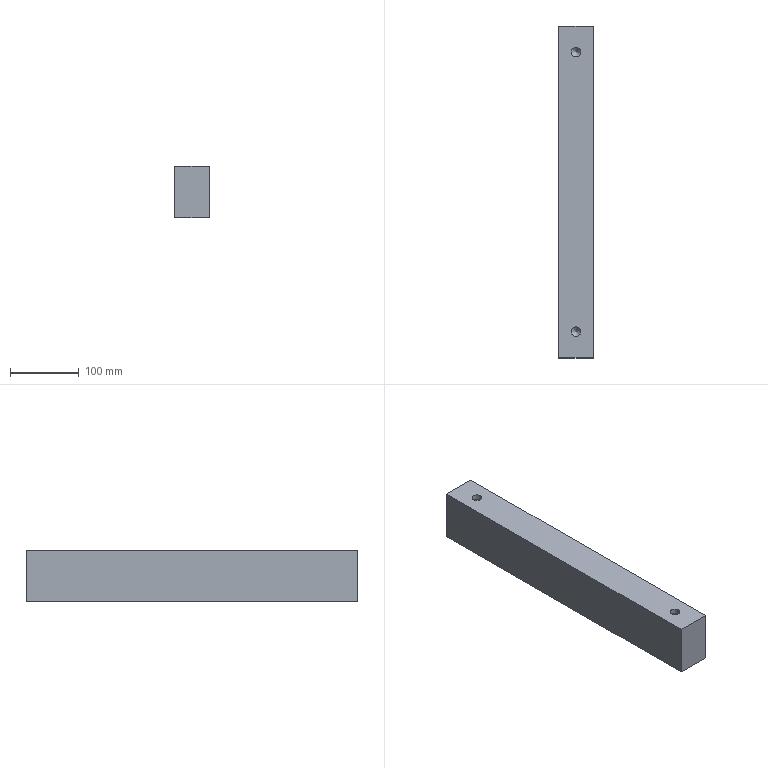Part | NX | features 3 2 | 1 solid | 10 faces | box 50 x 482.437 x 75.5 mm | volume 1817981 mm3 | plane 6 | cylinder 2 | cone 2 | commonest cylinder face diameters 14.1 x2
STEP:
#1=CARTESIAN_POINT('',(57.05,203.218,256.5));
#2=VERTEX_POINT('',#1);
#3=CARTESIAN_POINT('',(50.,203.218,256.5));
#4=DIRECTION('',(0.,0.,-1.));
#5=DIRECTION('',(1.,0.,0.));
#6=AXIS2_PLACEMENT_3D('',#3,#4,#5);
#7=CIRCLE('',#6,7.05);
#8=EDGE_CURVE('',#2,#2,#7,.T.);
#9=ORIENTED_EDGE('',*,*,#8,.T.);
#10=EDGE_LOOP('',(#9));
#11=FACE_BOUND('',#10,.T.);
#12=CARTESIAN_POINT('',(75.,241.218,256.5));
#13=VERTEX_POINT('',#12);
#14=CARTESIAN_POINT('',(75.,-241.218,256.5));
#15=VERTEX_POINT('',#14);
#16=CARTESIAN_POINT('',(75.,193.,256.5));
#17=DIRECTION('',(0.,-1.,0.));
#18=VECTOR('',#17,1000.);
#19=LINE('',#16,#18);
#20=EDGE_CURVE('',#13,#15,#19,.T.);
#21=ORIENTED_EDGE('',*,*,#20,.F.);
#22=CARTESIAN_POINT('',(25.,241.218,256.5));
#23=VERTEX_POINT('',#22);
#24=CARTESIAN_POINT('',(2065.,241.218,256.5));
#25=DIRECTION('',(1.,0.,0.));
#26=VECTOR('',#25,1000.);
#27=LINE('',#24,#26);
#28=EDGE_CURVE('',#23,#13,#27,.T.);
#29=ORIENTED_EDGE('',*,*,#28,.F.);
#30=CARTESIAN_POINT('',(25.,-241.218,256.5));
#31=VERTEX_POINT('',#30);
#32=CARTESIAN_POINT('',(25.,193.,256.5));
#33=DIRECTION('',(0.,1.,0.));
#34=VECTOR('',#33,1000.);
#35=LINE('',#32,#34);
#36=EDGE_CURVE('',#31,#23,#35,.T.);
#37=ORIENTED_EDGE('',*,*,#36,.F.);
#38=CARTESIAN_POINT('',(2065.,-241.218,256.5));
#39=DIRECTION('',(1.,0.,0.));
#40=VECTOR('',#39,1000.);
#41=LINE('',#38,#40);
#42=EDGE_CURVE('',#31,#15,#41,.T.);
#43=ORIENTED_EDGE('',*,*,#42,.T.);
#44=EDGE_LOOP('',(#21,#29,#37,#43));
#45=FACE_BOUND('',#44,.T.);
#46=CARTESIAN_POINT('',(57.05,-203.218,256.5));
#47=VERTEX_POINT('',#46);
#48=CARTESIAN_POINT('',(50.,-203.218,256.5));
#49=DIRECTION('',(0.,0.,-1.));
#50=DIRECTION('',(1.,0.,0.));
#51=AXIS2_PLACEMENT_3D('',#48,#49,#50);
#52=CIRCLE('',#51,7.05);
#53=EDGE_CURVE('',#47,#47,#52,.T.);
#54=ORIENTED_EDGE('',*,*,#53,.T.);
#55=EDGE_LOOP('',(#54));
#56=FACE_BOUND('',#55,.T.);
#57=CARTESIAN_POINT('',(2065.,0.,256.5));
#58=DIRECTION('',(0.,0.,1.));
#59=DIRECTION('',(-1.,0.,0.));
#60=AXIS2_PLACEMENT_3D('',#57,#58,#59);
#61=PLANE('',#60);
#62=ADVANCED_FACE('',(#11,#45,#56),#61,.T.);
#63=ORIENTED_EDGE('',*,*,#36,.T.);
#64=CARTESIAN_POINT('',(25.,241.218,181.));
#65=VERTEX_POINT('',#64);
#66=CARTESIAN_POINT('',(25.,241.218,-1.5));
#67=DIRECTION('',(0.,0.,1.));
#68=VECTOR('',#67,1000.);
#69=LINE('',#66,#68);
#70=EDGE_CURVE('',#65,#23,#69,.T.);
#71=ORIENTED_EDGE('',*,*,#70,.F.);
#72=CARTESIAN_POINT('',(25.,-241.218,181.));
#73=VERTEX_POINT('',#72);
#74=CARTESIAN_POINT('',(25.,193.,181.));
#75=DIRECTION('',(0.,-1.,0.));
#76=VECTOR('',#75,1000.);
#77=LINE('',#74,#76);
#78=EDGE_CURVE('',#65,#73,#77,.T.);
#79=ORIENTED_EDGE('',*,*,#78,.T.);
#80=CARTESIAN_POINT('',(25.,-241.218,-1.5));
#81=DIRECTION('',(0.,0.,1.));
#82=VECTOR('',#81,1000.);
#83=LINE('',#80,#82);
#84=EDGE_CURVE('',#73,#31,#83,.T.);
#85=ORIENTED_EDGE('',*,*,#84,.T.);
#86=EDGE_LOOP('',(#63,#71,#79,#85));
#87=FACE_BOUND('',#86,.T.);
#88=CARTESIAN_POINT('',(25.,193.,-1.5));
#89=DIRECTION('',(-1.,0.,0.));
#90=DIRECTION('',(0.,0.,-1.));
#91=AXIS2_PLACEMENT_3D('',#88,#89,#90);
#92=PLANE('',#91);
#93=ADVANCED_FACE('',(#87),#92,.T.);
#94=CARTESIAN_POINT('',(75.,-241.218,181.));
#95=VERTEX_POINT('',#94);
#96=CARTESIAN_POINT('',(75.,241.218,181.));
#97=VERTEX_POINT('',#96);
#98=CARTESIAN_POINT('',(75.,193.,181.));
#99=DIRECTION('',(0.,1.,0.));
#100=VECTOR('',#99,1000.);
#101=LINE('',#98,#100);
#102=EDGE_CURVE('',#95,#97,#101,.T.);
#103=ORIENTED_EDGE('',*,*,#102,.T.);
#104=CARTESIAN_POINT('',(75.,241.218,-1.5));
#105=DIRECTION('',(0.,0.,-1.));
#106=VECTOR('',#105,1000.);
#107=LINE('',#104,#106);
#108=EDGE_CURVE('',#13,#97,#107,.T.);
#109=ORIENTED_EDGE('',*,*,#108,.F.);
#110=ORIENTED_EDGE('',*,*,#20,.T.);
#111=CARTESIAN_POINT('',(75.,-241.218,-1.5));
#112=DIRECTION('',(0.,0.,-1.));
#113=VECTOR('',#112,1000.);
#114=LINE('',#111,#113);
#115=EDGE_CURVE('',#15,#95,#114,.T.);
#116=ORIENTED_EDGE('',*,*,#115,.T.);
#117=EDGE_LOOP('',(#103,#109,#110,#116));
#118=FACE_BOUND('',#117,.T.);
#119=CARTESIAN_POINT('',(75.,193.,-1.5));
#120=DIRECTION('',(1.,0.,0.));
#121=DIRECTION('',(0.,0.,1.));
#122=AXIS2_PLACEMENT_3D('',#119,#120,#121);
#123=PLANE('',#122);
#124=ADVANCED_FACE('',(#118),#123,.T.);
#125=ORIENTED_EDGE('',*,*,#78,.F.);
#126=CARTESIAN_POINT('',(1295.,241.218,181.));
#127=DIRECTION('',(-1.,0.,0.));
#128=VECTOR('',#127,1000.);
#129=LINE('',#126,#128);
#130=EDGE_CURVE('',#97,#65,#129,.T.);
#131=ORIENTED_EDGE('',*,*,#130,.F.);
#132=ORIENTED_EDGE('',*,*,#102,.F.);
#133=CARTESIAN_POINT('',(1295.,-241.218,181.));
#134=DIRECTION('',(-1.,0.,0.));
#135=VECTOR('',#134,1000.);
#136=LINE('',#133,#135);
#137=EDGE_CURVE('',#95,#73,#136,.T.);
#138=ORIENTED_EDGE('',*,*,#137,.T.);
#139=EDGE_LOOP('',(#125,#131,#132,#138));
#140=FACE_BOUND('',#139,.T.);
#141=CARTESIAN_POINT('',(1295.,193.,181.));
#142=DIRECTION('',(0.,0.,-1.));
#143=DIRECTION('',(-1.,0.,0.));
#144=AXIS2_PLACEMENT_3D('',#141,#142,#143);
#145=PLANE('',#144);
#146=ADVANCED_FACE('',(#140),#145,.T.);
#147=ORIENTED_EDGE('',*,*,#42,.F.);
#148=ORIENTED_EDGE('',*,*,#84,.F.);
#149=ORIENTED_EDGE('',*,*,#137,.F.);
#150=ORIENTED_EDGE('',*,*,#115,.F.);
#151=EDGE_LOOP('',(#147,#148,#149,#150));
#152=FACE_BOUND('',#151,.T.);
#153=CARTESIAN_POINT('',(-126.629,-241.218,0.));
#154=DIRECTION('',(0.,-1.,0.));
#155=DIRECTION('',(0.,0.,1.));
#156=AXIS2_PLACEMENT_3D('',#153,#154,#155);
#157=PLANE('',#156);
#158=ADVANCED_FACE('',(#152),#157,.T.);
#159=ORIENTED_EDGE('',*,*,#28,.T.);
#160=ORIENTED_EDGE('',*,*,#108,.T.);
#161=ORIENTED_EDGE('',*,*,#130,.T.);
#162=ORIENTED_EDGE('',*,*,#70,.T.);
#163=EDGE_LOOP('',(#159,#160,#161,#162));
#164=FACE_BOUND('',#163,.T.);
#165=CARTESIAN_POINT('',(-126.629,241.218,0.));
#166=DIRECTION('',(0.,1.,0.));
#167=DIRECTION('',(0.,0.,1.));
#168=AXIS2_PLACEMENT_3D('',#165,#166,#167);
#169=PLANE('',#168);
#170=ADVANCED_FACE('',(#164),#169,.T.);
#171=CARTESIAN_POINT('',(42.95,203.218,248.55));
#172=VERTEX_POINT('',#171);
#173=CARTESIAN_POINT('',(50.,203.218,248.55));
#174=DIRECTION('',(0.,0.,-1.));
#175=DIRECTION('',(-1.,0.,0.));
#176=AXIS2_PLACEMENT_3D('',#173,#174,#175);
#177=CIRCLE('',#176,7.05);
#178=EDGE_CURVE('',#172,#172,#177,.T.);
#179=ORIENTED_EDGE('',*,*,#178,.T.);
#180=EDGE_LOOP('',(#179));
#181=FACE_BOUND('',#180,.T.);
#182=ORIENTED_EDGE('',*,*,#8,.F.);
#183=EDGE_LOOP('',(#182));
#184=FACE_BOUND('',#183,.T.);
#185=CARTESIAN_POINT('',(50.,203.218,256.5));
#186=DIRECTION('',(0.,0.,-1.));
#187=DIRECTION('',(-1.,0.,0.));
#188=AXIS2_PLACEMENT_3D('',#185,#186,#187);
#189=CYLINDRICAL_SURFACE('',#188,7.05);
#190=ADVANCED_FACE('',(#181,#184),#189,.F.);
#191=CARTESIAN_POINT('',(50.,203.218,241.5));
#192=VERTEX_POINT('',#191);
#193=VERTEX_LOOP('',#192);
#194=FACE_BOUND('',#193,.T.);
#195=ORIENTED_EDGE('',*,*,#178,.F.);
#196=EDGE_LOOP('',(#195));
#197=FACE_BOUND('',#196,.T.);
#198=CARTESIAN_POINT('',(50.,203.218,248.55));
#199=DIRECTION('',(0.,0.,1.));
#200=DIRECTION('',(-1.,0.,0.));
#201=AXIS2_PLACEMENT_3D('',#198,#199,#200);
#202=CONICAL_SURFACE('',#201,7.05,0.7854);
#203=ADVANCED_FACE('',(#194,#197),#202,.F.);
#204=CARTESIAN_POINT('',(42.95,-203.218,248.55));
#205=VERTEX_POINT('',#204);
#206=CARTESIAN_POINT('',(50.,-203.218,248.55));
#207=DIRECTION('',(0.,0.,-1.));
#208=DIRECTION('',(-1.,0.,0.));
#209=AXIS2_PLACEMENT_3D('',#206,#207,#208);
#210=CIRCLE('',#209,7.05);
#211=EDGE_CURVE('',#205,#205,#210,.T.);
#212=ORIENTED_EDGE('',*,*,#211,.T.);
#213=EDGE_LOOP('',(#212));
#214=FACE_BOUND('',#213,.T.);
#215=ORIENTED_EDGE('',*,*,#53,.F.);
#216=EDGE_LOOP('',(#215));
#217=FACE_BOUND('',#216,.T.);
#218=CARTESIAN_POINT('',(50.,-203.218,256.5));
#219=DIRECTION('',(0.,0.,-1.));
#220=DIRECTION('',(-1.,0.,0.));
#221=AXIS2_PLACEMENT_3D('',#218,#219,#220);
#222=CYLINDRICAL_SURFACE('',#221,7.05);
#223=ADVANCED_FACE('',(#214,#217),#222,.F.);
#224=CARTESIAN_POINT('',(50.,-203.218,241.5));
#225=VERTEX_POINT('',#224);
#226=VERTEX_LOOP('',#225);
#227=FACE_BOUND('',#226,.T.);
#228=ORIENTED_EDGE('',*,*,#211,.F.);
#229=EDGE_LOOP('',(#228));
#230=FACE_BOUND('',#229,.T.);
#231=CARTESIAN_POINT('',(50.,-203.218,248.55));
#232=DIRECTION('',(0.,0.,1.));
#233=DIRECTION('',(-1.,0.,0.));
#234=AXIS2_PLACEMENT_3D('',#231,#232,#233);
#235=CONICAL_SURFACE('',#234,7.05,0.7854);
#236=ADVANCED_FACE('',(#227,#230),#235,.F.);
#237=CLOSED_SHELL('',(#62,#93,#124,#146,#158,#170,#190,#203,#223,#236));
#238=MANIFOLD_SOLID_BREP('',#237);
#239=(LENGTH_UNIT()NAMED_UNIT(*)SI_UNIT(.MILLI.,.METRE.));
#240=UNCERTAINTY_MEASURE_WITH_UNIT(LENGTH_MEASURE(0.00001),#239,'','');
#241=(NAMED_UNIT(*)PLANE_ANGLE_UNIT()SI_UNIT($,.RADIAN.));
#242=(NAMED_UNIT(*)SI_UNIT($,.STERADIAN.)SOLID_ANGLE_UNIT());
#243=(GEOMETRIC_REPRESENTATION_CONTEXT(3)GLOBAL_UNCERTAINTY_ASSIGNED_CONTEXT((#240))GLOBAL_UNIT_ASSIGNED_CONTEXT((#239,#241,#242))REPRESENTATION_CONTEXT('',''));
#244=ADVANCED_BREP_SHAPE_REPRESENTATION('',(#238),#243);